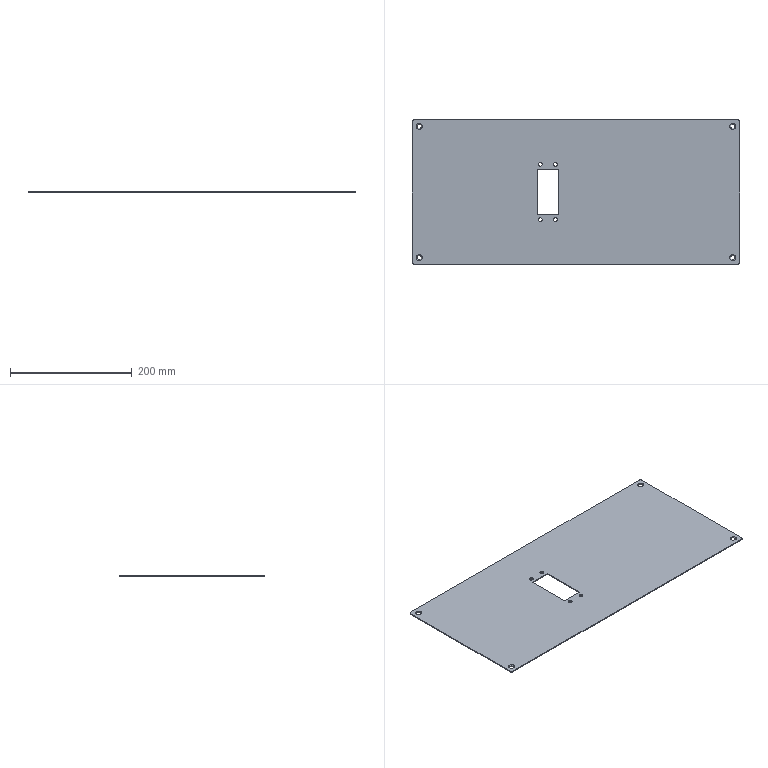Part | SolidWorks | features HoleWzd 2, Cut 1, Extrusion 1, Fillet 1, ICE 1 | 1 solid | 36 faces | box 538.2 x 238 x 1.5 mm | volume 187659 mm3 | cylinder 18 | plane 10 | cone 8 | commonest cylinder face diameters 6.4 x8 7.1 x6 6 x4
STEP:
#1=CARTESIAN_POINT('',(-25.62,94.068,-1.5));
#2=VERTEX_POINT('',#1);
#3=CARTESIAN_POINT('',(-19.22,94.068,-1.5));
#4=VERTEX_POINT('',#3);
#5=CARTESIAN_POINT('',(-22.42,94.068,-1.5));
#6=DIRECTION('',(0.,0.,1.));
#7=DIRECTION('',(1.,0.,0.));
#8=AXIS2_PLACEMENT_3D('',#5,#6,#7);
#9=CIRCLE('',#8,3.2);
#10=EDGE_CURVE('',#2,#4,#9,.T.);
#11=ORIENTED_EDGE('',*,*,#10,.F.);
#12=CARTESIAN_POINT('',(-25.62,94.068,0.));
#13=VERTEX_POINT('',#12);
#14=CARTESIAN_POINT('',(-25.62,94.068,-1.5));
#15=DIRECTION('',(0.,0.,1.));
#16=VECTOR('',#15,1000.);
#17=LINE('',#14,#16);
#18=EDGE_CURVE('',#2,#13,#17,.T.);
#19=ORIENTED_EDGE('',*,*,#18,.T.);
#20=CARTESIAN_POINT('',(-19.22,94.068,0.));
#21=VERTEX_POINT('',#20);
#22=CARTESIAN_POINT('',(-22.42,94.068,0.));
#23=DIRECTION('',(0.,0.,1.));
#24=DIRECTION('',(1.,0.,0.));
#25=AXIS2_PLACEMENT_3D('',#22,#23,#24);
#26=CIRCLE('',#25,3.2);
#27=EDGE_CURVE('',#13,#21,#26,.T.);
#28=ORIENTED_EDGE('',*,*,#27,.T.);
#29=CARTESIAN_POINT('',(-19.22,94.068,-1.5));
#30=DIRECTION('',(0.,0.,1.));
#31=VECTOR('',#30,1000.);
#32=LINE('',#29,#31);
#33=EDGE_CURVE('',#4,#21,#32,.T.);
#34=ORIENTED_EDGE('',*,*,#33,.F.);
#35=EDGE_LOOP('',(#11,#19,#28,#34));
#36=FACE_OUTER_BOUND('',#35,.T.);
#37=CARTESIAN_POINT('',(-22.42,94.068,-1.5));
#38=DIRECTION('',(0.,0.,1.));
#39=DIRECTION('',(1.,0.,0.));
#40=AXIS2_PLACEMENT_3D('',#37,#38,#39);
#41=CYLINDRICAL_SURFACE('',#40,3.2);
#42=ADVANCED_FACE('',(#36),#41,.F.);
#43=CARTESIAN_POINT('',(-0.6198,185.068,-1.5));
#44=VERTEX_POINT('',#43);
#45=CARTESIAN_POINT('',(5.78,185.068,-1.5));
#46=VERTEX_POINT('',#45);
#47=CARTESIAN_POINT('',(2.58,185.068,-1.5));
#48=DIRECTION('',(0.,0.,1.));
#49=DIRECTION('',(1.,0.,0.));
#50=AXIS2_PLACEMENT_3D('',#47,#48,#49);
#51=CIRCLE('',#50,3.2);
#52=EDGE_CURVE('',#44,#46,#51,.T.);
#53=ORIENTED_EDGE('',*,*,#52,.F.);
#54=CARTESIAN_POINT('',(-0.6198,185.068,0.));
#55=VERTEX_POINT('',#54);
#56=CARTESIAN_POINT('',(-0.6198,185.068,-1.5));
#57=DIRECTION('',(0.,0.,1.));
#58=VECTOR('',#57,1000.);
#59=LINE('',#56,#58);
#60=EDGE_CURVE('',#44,#55,#59,.T.);
#61=ORIENTED_EDGE('',*,*,#60,.T.);
#62=CARTESIAN_POINT('',(5.78,185.068,0.));
#63=VERTEX_POINT('',#62);
#64=CARTESIAN_POINT('',(2.58,185.068,0.));
#65=DIRECTION('',(0.,0.,1.));
#66=DIRECTION('',(1.,0.,0.));
#67=AXIS2_PLACEMENT_3D('',#64,#65,#66);
#68=CIRCLE('',#67,3.2);
#69=EDGE_CURVE('',#55,#63,#68,.T.);
#70=ORIENTED_EDGE('',*,*,#69,.T.);
#71=CARTESIAN_POINT('',(5.78,185.068,-1.5));
#72=DIRECTION('',(0.,0.,1.));
#73=VECTOR('',#72,1000.);
#74=LINE('',#71,#73);
#75=EDGE_CURVE('',#46,#63,#74,.T.);
#76=ORIENTED_EDGE('',*,*,#75,.F.);
#77=EDGE_LOOP('',(#53,#61,#70,#76));
#78=FACE_OUTER_BOUND('',#77,.T.);
#79=CARTESIAN_POINT('',(2.58,185.068,-1.5));
#80=DIRECTION('',(0.,0.,1.));
#81=DIRECTION('',(1.,0.,0.));
#82=AXIS2_PLACEMENT_3D('',#79,#80,#81);
#83=CYLINDRICAL_SURFACE('',#82,3.2);
#84=ADVANCED_FACE('',(#78),#83,.F.);
#85=CARTESIAN_POINT('',(-25.62,185.068,-1.5));
#86=VERTEX_POINT('',#85);
#87=CARTESIAN_POINT('',(-19.22,185.068,-1.5));
#88=VERTEX_POINT('',#87);
#89=CARTESIAN_POINT('',(-22.42,185.068,-1.5));
#90=DIRECTION('',(0.,0.,1.));
#91=DIRECTION('',(1.,0.,0.));
#92=AXIS2_PLACEMENT_3D('',#89,#90,#91);
#93=CIRCLE('',#92,3.2);
#94=EDGE_CURVE('',#86,#88,#93,.T.);
#95=ORIENTED_EDGE('',*,*,#94,.F.);
#96=CARTESIAN_POINT('',(-25.62,185.068,0.));
#97=VERTEX_POINT('',#96);
#98=CARTESIAN_POINT('',(-25.62,185.068,-1.5));
#99=DIRECTION('',(0.,0.,1.));
#100=VECTOR('',#99,1000.);
#101=LINE('',#98,#100);
#102=EDGE_CURVE('',#86,#97,#101,.T.);
#103=ORIENTED_EDGE('',*,*,#102,.T.);
#104=CARTESIAN_POINT('',(-19.22,185.068,0.));
#105=VERTEX_POINT('',#104);
#106=CARTESIAN_POINT('',(-22.42,185.068,0.));
#107=DIRECTION('',(0.,0.,1.));
#108=DIRECTION('',(1.,0.,0.));
#109=AXIS2_PLACEMENT_3D('',#106,#107,#108);
#110=CIRCLE('',#109,3.2);
#111=EDGE_CURVE('',#97,#105,#110,.T.);
#112=ORIENTED_EDGE('',*,*,#111,.T.);
#113=CARTESIAN_POINT('',(-19.22,185.068,-1.5));
#114=DIRECTION('',(0.,0.,1.));
#115=VECTOR('',#114,1000.);
#116=LINE('',#113,#115);
#117=EDGE_CURVE('',#88,#105,#116,.T.);
#118=ORIENTED_EDGE('',*,*,#117,.F.);
#119=EDGE_LOOP('',(#95,#103,#112,#118));
#120=FACE_OUTER_BOUND('',#119,.T.);
#121=CARTESIAN_POINT('',(-22.42,185.068,-1.5));
#122=DIRECTION('',(0.,0.,1.));
#123=DIRECTION('',(1.,0.,0.));
#124=AXIS2_PLACEMENT_3D('',#121,#122,#123);
#125=CYLINDRICAL_SURFACE('',#124,3.2);
#126=ADVANCED_FACE('',(#120),#125,.F.);
#127=CARTESIAN_POINT('',(-0.6198,94.068,-1.5));
#128=VERTEX_POINT('',#127);
#129=CARTESIAN_POINT('',(5.78,94.068,-1.5));
#130=VERTEX_POINT('',#129);
#131=CARTESIAN_POINT('',(2.58,94.068,-1.5));
#132=DIRECTION('',(0.,0.,1.));
#133=DIRECTION('',(1.,0.,0.));
#134=AXIS2_PLACEMENT_3D('',#131,#132,#133);
#135=CIRCLE('',#134,3.2);
#136=EDGE_CURVE('',#128,#130,#135,.T.);
#137=ORIENTED_EDGE('',*,*,#136,.F.);
#138=CARTESIAN_POINT('',(-0.6198,94.068,0.));
#139=VERTEX_POINT('',#138);
#140=CARTESIAN_POINT('',(-0.6198,94.068,-1.5));
#141=DIRECTION('',(0.,0.,1.));
#142=VECTOR('',#141,1000.);
#143=LINE('',#140,#142);
#144=EDGE_CURVE('',#128,#139,#143,.T.);
#145=ORIENTED_EDGE('',*,*,#144,.T.);
#146=CARTESIAN_POINT('',(5.78,94.068,0.));
#147=VERTEX_POINT('',#146);
#148=CARTESIAN_POINT('',(2.58,94.068,0.));
#149=DIRECTION('',(0.,0.,1.));
#150=DIRECTION('',(1.,0.,0.));
#151=AXIS2_PLACEMENT_3D('',#148,#149,#150);
#152=CIRCLE('',#151,3.2);
#153=EDGE_CURVE('',#139,#147,#152,.T.);
#154=ORIENTED_EDGE('',*,*,#153,.T.);
#155=CARTESIAN_POINT('',(5.78,94.068,-1.5));
#156=DIRECTION('',(0.,0.,1.));
#157=VECTOR('',#156,1000.);
#158=LINE('',#155,#157);
#159=EDGE_CURVE('',#130,#147,#158,.T.);
#160=ORIENTED_EDGE('',*,*,#159,.F.);
#161=EDGE_LOOP('',(#137,#145,#154,#160));
#162=FACE_OUTER_BOUND('',#161,.T.);
#163=CARTESIAN_POINT('',(2.58,94.068,-1.5));
#164=DIRECTION('',(0.,0.,1.));
#165=DIRECTION('',(1.,0.,0.));
#166=AXIS2_PLACEMENT_3D('',#163,#164,#165);
#167=CYLINDRICAL_SURFACE('',#166,3.2);
#168=ADVANCED_FACE('',(#162),#167,.F.);
#169=CARTESIAN_POINT('',(291.03,247.568,-1.4));
#170=VERTEX_POINT('',#169);
#171=CARTESIAN_POINT('',(298.13,247.568,-1.4));
#172=VERTEX_POINT('',#171);
#173=CARTESIAN_POINT('',(294.58,247.568,-1.4));
#174=DIRECTION('',(0.,0.,1.));
#175=DIRECTION('',(1.,0.,0.));
#176=AXIS2_PLACEMENT_3D('',#173,#174,#175);
#177=CIRCLE('',#176,3.55);
#178=EDGE_CURVE('',#170,#172,#177,.T.);
#179=ORIENTED_EDGE('',*,*,#178,.F.);
#180=CARTESIAN_POINT('',(289.63,247.568,0.));
#181=VERTEX_POINT('',#180);
#182=CARTESIAN_POINT('',(289.63,247.568,0.));
#183=DIRECTION('',(-0.7071,0.,0.7071));
#184=VECTOR('',#183,1000.);
#185=LINE('',#182,#184);
#186=EDGE_CURVE('',#170,#181,#185,.T.);
#187=ORIENTED_EDGE('',*,*,#186,.T.);
#188=CARTESIAN_POINT('',(299.53,247.568,0.));
#189=VERTEX_POINT('',#188);
#190=CARTESIAN_POINT('',(294.58,247.568,0.));
#191=DIRECTION('',(0.,0.,1.));
#192=DIRECTION('',(1.,0.,0.));
#193=AXIS2_PLACEMENT_3D('',#190,#191,#192);
#194=CIRCLE('',#193,4.95);
#195=EDGE_CURVE('',#181,#189,#194,.T.);
#196=ORIENTED_EDGE('',*,*,#195,.T.);
#197=CARTESIAN_POINT('',(299.53,247.568,0.));
#198=DIRECTION('',(0.7071,0.,0.7071));
#199=VECTOR('',#198,1000.);
#200=LINE('',#197,#199);
#201=EDGE_CURVE('',#172,#189,#200,.T.);
#202=ORIENTED_EDGE('',*,*,#201,.F.);
#203=EDGE_LOOP('',(#179,#187,#196,#202));
#204=FACE_OUTER_BOUND('',#203,.T.);
#205=CARTESIAN_POINT('',(294.58,247.568,0.));
#206=DIRECTION('',(0.,0.,1.));
#207=DIRECTION('',(1.,0.,0.));
#208=AXIS2_PLACEMENT_3D('',#205,#206,#207);
#209=CONICAL_SURFACE('',#208,4.95,0.7854);
#210=ADVANCED_FACE('',(#204),#209,.F.);
#211=CARTESIAN_POINT('',(291.03,247.568,-1.5));
#212=VERTEX_POINT('',#211);
#213=CARTESIAN_POINT('',(298.13,247.568,-1.5));
#214=VERTEX_POINT('',#213);
#215=CARTESIAN_POINT('',(294.58,247.568,-1.5));
#216=DIRECTION('',(0.,0.,1.));
#217=DIRECTION('',(1.,0.,0.));
#218=AXIS2_PLACEMENT_3D('',#215,#216,#217);
#219=CIRCLE('',#218,3.55);
#220=EDGE_CURVE('',#212,#214,#219,.T.);
#221=ORIENTED_EDGE('',*,*,#220,.F.);
#222=CARTESIAN_POINT('',(291.03,247.568,0.));
#223=DIRECTION('',(0.,0.,1.));
#224=VECTOR('',#223,1000.);
#225=LINE('',#222,#224);
#226=EDGE_CURVE('',#212,#170,#225,.T.);
#227=ORIENTED_EDGE('',*,*,#226,.T.);
#228=ORIENTED_EDGE('',*,*,#178,.T.);
#229=CARTESIAN_POINT('',(298.13,247.568,0.));
#230=DIRECTION('',(0.,0.,1.));
#231=VECTOR('',#230,1000.);
#232=LINE('',#229,#231);
#233=EDGE_CURVE('',#214,#172,#232,.T.);
#234=ORIENTED_EDGE('',*,*,#233,.F.);
#235=EDGE_LOOP('',(#221,#227,#228,#234));
#236=FACE_OUTER_BOUND('',#235,.T.);
#237=CARTESIAN_POINT('',(294.58,247.568,0.));
#238=DIRECTION('',(0.,0.,1.));
#239=DIRECTION('',(1.,0.,0.));
#240=AXIS2_PLACEMENT_3D('',#237,#238,#239);
#241=CYLINDRICAL_SURFACE('',#240,3.55);
#242=ADVANCED_FACE('',(#236),#241,.F.);
#243=CARTESIAN_POINT('',(291.03,31.568,-1.4));
#244=VERTEX_POINT('',#243);
#245=CARTESIAN_POINT('',(298.13,31.568,-1.4));
#246=VERTEX_POINT('',#245);
#247=CARTESIAN_POINT('',(294.58,31.568,-1.4));
#248=DIRECTION('',(0.,0.,1.));
#249=DIRECTION('',(1.,0.,0.));
#250=AXIS2_PLACEMENT_3D('',#247,#248,#249);
#251=CIRCLE('',#250,3.55);
#252=EDGE_CURVE('',#244,#246,#251,.T.);
#253=ORIENTED_EDGE('',*,*,#252,.F.);
#254=CARTESIAN_POINT('',(289.63,31.568,0.));
#255=VERTEX_POINT('',#254);
#256=CARTESIAN_POINT('',(289.63,31.568,0.));
#257=DIRECTION('',(-0.7071,0.,0.7071));
#258=VECTOR('',#257,1000.);
#259=LINE('',#256,#258);
#260=EDGE_CURVE('',#244,#255,#259,.T.);
#261=ORIENTED_EDGE('',*,*,#260,.T.);
#262=CARTESIAN_POINT('',(299.53,31.568,0.));
#263=VERTEX_POINT('',#262);
#264=CARTESIAN_POINT('',(294.58,31.568,0.));
#265=DIRECTION('',(0.,0.,1.));
#266=DIRECTION('',(1.,0.,0.));
#267=AXIS2_PLACEMENT_3D('',#264,#265,#266);
#268=CIRCLE('',#267,4.95);
#269=EDGE_CURVE('',#255,#263,#268,.T.);
#270=ORIENTED_EDGE('',*,*,#269,.T.);
#271=CARTESIAN_POINT('',(299.53,31.568,0.));
#272=DIRECTION('',(0.7071,0.,0.7071));
#273=VECTOR('',#272,1000.);
#274=LINE('',#271,#273);
#275=EDGE_CURVE('',#246,#263,#274,.T.);
#276=ORIENTED_EDGE('',*,*,#275,.F.);
#277=EDGE_LOOP('',(#253,#261,#270,#276));
#278=FACE_OUTER_BOUND('',#277,.T.);
#279=CARTESIAN_POINT('',(294.58,31.568,0.));
#280=DIRECTION('',(0.,0.,1.));
#281=DIRECTION('',(1.,0.,0.));
#282=AXIS2_PLACEMENT_3D('',#279,#280,#281);
#283=CONICAL_SURFACE('',#282,4.95,0.7854);
#284=ADVANCED_FACE('',(#278),#283,.F.);
#285=CARTESIAN_POINT('',(291.03,31.568,-1.5));
#286=VERTEX_POINT('',#285);
#287=CARTESIAN_POINT('',(298.13,31.568,-1.5));
#288=VERTEX_POINT('',#287);
#289=CARTESIAN_POINT('',(294.58,31.568,-1.5));
#290=DIRECTION('',(0.,0.,1.));
#291=DIRECTION('',(1.,0.,0.));
#292=AXIS2_PLACEMENT_3D('',#289,#290,#291);
#293=CIRCLE('',#292,3.55);
#294=EDGE_CURVE('',#286,#288,#293,.T.);
#295=ORIENTED_EDGE('',*,*,#294,.F.);
#296=CARTESIAN_POINT('',(291.03,31.568,0.));
#297=DIRECTION('',(0.,0.,1.));
#298=VECTOR('',#297,1000.);
#299=LINE('',#296,#298);
#300=EDGE_CURVE('',#286,#244,#299,.T.);
#301=ORIENTED_EDGE('',*,*,#300,.T.);
#302=ORIENTED_EDGE('',*,*,#252,.T.);
#303=CARTESIAN_POINT('',(298.13,31.568,0.));
#304=DIRECTION('',(0.,0.,1.));
#305=VECTOR('',#304,1000.);
#306=LINE('',#303,#305);
#307=EDGE_CURVE('',#288,#246,#306,.T.);
#308=ORIENTED_EDGE('',*,*,#307,.F.);
#309=EDGE_LOOP('',(#295,#301,#302,#308));
#310=FACE_OUTER_BOUND('',#309,.T.);
#311=CARTESIAN_POINT('',(294.58,31.568,0.));
#312=DIRECTION('',(0.,0.,1.));
#313=DIRECTION('',(1.,0.,0.));
#314=AXIS2_PLACEMENT_3D('',#311,#312,#313);
#315=CYLINDRICAL_SURFACE('',#314,3.55);
#316=ADVANCED_FACE('',(#310),#315,.F.);
#317=CARTESIAN_POINT('',(-225.17,247.568,-1.4));
#318=VERTEX_POINT('',#317);
#319=CARTESIAN_POINT('',(-218.07,247.568,-1.4));
#320=VERTEX_POINT('',#319);
#321=CARTESIAN_POINT('',(-221.62,247.568,-1.4));
#322=DIRECTION('',(0.,0.,1.));
#323=DIRECTION('',(1.,0.,0.));
#324=AXIS2_PLACEMENT_3D('',#321,#322,#323);
#325=CIRCLE('',#324,3.55);
#326=EDGE_CURVE('',#318,#320,#325,.T.);
#327=ORIENTED_EDGE('',*,*,#326,.F.);
#328=CARTESIAN_POINT('',(-226.57,247.568,0.));
#329=VERTEX_POINT('',#328);
#330=CARTESIAN_POINT('',(-226.57,247.568,0.));
#331=DIRECTION('',(-0.7071,0.,0.7071));
#332=VECTOR('',#331,1000.);
#333=LINE('',#330,#332);
#334=EDGE_CURVE('',#318,#329,#333,.T.);
#335=ORIENTED_EDGE('',*,*,#334,.T.);
#336=CARTESIAN_POINT('',(-216.67,247.568,0.));
#337=VERTEX_POINT('',#336);
#338=CARTESIAN_POINT('',(-221.62,247.568,0.));
#339=DIRECTION('',(0.,0.,1.));
#340=DIRECTION('',(1.,0.,0.));
#341=AXIS2_PLACEMENT_3D('',#338,#339,#340);
#342=CIRCLE('',#341,4.95);
#343=EDGE_CURVE('',#329,#337,#342,.T.);
#344=ORIENTED_EDGE('',*,*,#343,.T.);
#345=CARTESIAN_POINT('',(-216.67,247.568,0.));
#346=DIRECTION('',(0.7071,0.,0.7071));
#347=VECTOR('',#346,1000.);
#348=LINE('',#345,#347);
#349=EDGE_CURVE('',#320,#337,#348,.T.);
#350=ORIENTED_EDGE('',*,*,#349,.F.);
#351=EDGE_LOOP('',(#327,#335,#344,#350));
#352=FACE_OUTER_BOUND('',#351,.T.);
#353=CARTESIAN_POINT('',(-221.62,247.568,0.));
#354=DIRECTION('',(0.,0.,1.));
#355=DIRECTION('',(1.,0.,0.));
#356=AXIS2_PLACEMENT_3D('',#353,#354,#355);
#357=CONICAL_SURFACE('',#356,4.95,0.7854);
#358=ADVANCED_FACE('',(#352),#357,.F.);
#359=CARTESIAN_POINT('',(-225.17,247.568,-1.5));
#360=VERTEX_POINT('',#359);
#361=CARTESIAN_POINT('',(-218.07,247.568,-1.5));
#362=VERTEX_POINT('',#361);
#363=CARTESIAN_POINT('',(-221.62,247.568,-1.5));
#364=DIRECTION('',(0.,0.,1.));
#365=DIRECTION('',(1.,0.,0.));
#366=AXIS2_PLACEMENT_3D('',#363,#364,#365);
#367=CIRCLE('',#366,3.55);
#368=EDGE_CURVE('',#360,#362,#367,.T.);
#369=ORIENTED_EDGE('',*,*,#368,.F.);
#370=CARTESIAN_POINT('',(-225.17,247.568,0.));
#371=DIRECTION('',(0.,0.,1.));
#372=VECTOR('',#371,1000.);
#373=LINE('',#370,#372);
#374=EDGE_CURVE('',#360,#318,#373,.T.);
#375=ORIENTED_EDGE('',*,*,#374,.T.);
#376=ORIENTED_EDGE('',*,*,#326,.T.);
#377=CARTESIAN_POINT('',(-218.07,247.568,0.));
#378=DIRECTION('',(0.,0.,1.));
#379=VECTOR('',#378,1000.);
#380=LINE('',#377,#379);
#381=EDGE_CURVE('',#362,#320,#380,.T.);
#382=ORIENTED_EDGE('',*,*,#381,.F.);
#383=EDGE_LOOP('',(#369,#375,#376,#382));
#384=FACE_OUTER_BOUND('',#383,.T.);
#385=CARTESIAN_POINT('',(-221.62,247.568,0.));
#386=DIRECTION('',(0.,0.,1.));
#387=DIRECTION('',(1.,0.,0.));
#388=AXIS2_PLACEMENT_3D('',#385,#386,#387);
#389=CYLINDRICAL_SURFACE('',#388,3.55);
#390=ADVANCED_FACE('',(#384),#389,.F.);
#391=CARTESIAN_POINT('',(-225.07,31.568,-1.5));
#392=VERTEX_POINT('',#391);
#393=CARTESIAN_POINT('',(-218.17,31.568,-1.5));
#394=VERTEX_POINT('',#393);
#395=CARTESIAN_POINT('',(-221.62,31.568,-1.5));
#396=DIRECTION('',(0.,0.,1.));
#397=DIRECTION('',(1.,0.,0.));
#398=AXIS2_PLACEMENT_3D('',#395,#396,#397);
#399=CIRCLE('',#398,3.45);
#400=EDGE_CURVE('',#392,#394,#399,.T.);
#401=ORIENTED_EDGE('',*,*,#400,.F.);
#402=CARTESIAN_POINT('',(-226.57,31.568,0.));
#403=VERTEX_POINT('',#402);
#404=CARTESIAN_POINT('',(-226.57,31.568,0.));
#405=DIRECTION('',(-0.7071,0.,0.7071));
#406=VECTOR('',#405,1000.);
#407=LINE('',#404,#406);
#408=EDGE_CURVE('',#392,#403,#407,.T.);
#409=ORIENTED_EDGE('',*,*,#408,.T.);
#410=CARTESIAN_POINT('',(-216.67,31.568,0.));
#411=VERTEX_POINT('',#410);
#412=CARTESIAN_POINT('',(-221.62,31.568,0.));
#413=DIRECTION('',(0.,0.,1.));
#414=DIRECTION('',(1.,0.,0.));
#415=AXIS2_PLACEMENT_3D('',#412,#413,#414);
#416=CIRCLE('',#415,4.95);
#417=EDGE_CURVE('',#403,#411,#416,.T.);
#418=ORIENTED_EDGE('',*,*,#417,.T.);
#419=CARTESIAN_POINT('',(-216.67,31.568,0.));
#420=DIRECTION('',(0.7071,0.,0.7071));
#421=VECTOR('',#420,1000.);
#422=LINE('',#419,#421);
#423=EDGE_CURVE('',#394,#411,#422,.T.);
#424=ORIENTED_EDGE('',*,*,#423,.F.);
#425=EDGE_LOOP('',(#401,#409,#418,#424));
#426=FACE_OUTER_BOUND('',#425,.T.);
#427=CARTESIAN_POINT('',(-221.62,31.568,0.));
#428=DIRECTION('',(0.,0.,1.));
#429=DIRECTION('',(1.,0.,0.));
#430=AXIS2_PLACEMENT_3D('',#427,#428,#429);
#431=CONICAL_SURFACE('',#430,4.95,0.7854);
#432=ADVANCED_FACE('',(#426),#431,.F.);
#433=CARTESIAN_POINT('',(-232.62,255.568,-1.5));
#434=VERTEX_POINT('',#433);
#435=CARTESIAN_POINT('',(-232.62,23.568,-1.5));
#436=VERTEX_POINT('',#435);
#437=CARTESIAN_POINT('',(-232.62,258.568,-1.5));
#438=DIRECTION('',(0.,-1.,0.));
#439=VECTOR('',#438,1000.);
#440=LINE('',#437,#439);
#441=EDGE_CURVE('',#434,#436,#440,.T.);
#442=ORIENTED_EDGE('',*,*,#441,.T.);
#443=CARTESIAN_POINT('',(-232.62,23.568,0.));
#444=VERTEX_POINT('',#443);
#445=CARTESIAN_POINT('',(-232.62,23.568,-1.5));
#446=DIRECTION('',(0.,0.,1.));
#447=VECTOR('',#446,1000.);
#448=LINE('',#445,#447);
#449=EDGE_CURVE('',#436,#444,#448,.T.);
#450=ORIENTED_EDGE('',*,*,#449,.T.);
#451=CARTESIAN_POINT('',(-232.62,255.568,0.));
#452=VERTEX_POINT('',#451);
#453=CARTESIAN_POINT('',(-232.62,258.568,0.));
#454=DIRECTION('',(0.,-1.,0.));
#455=VECTOR('',#454,1000.);
#456=LINE('',#453,#455);
#457=EDGE_CURVE('',#452,#444,#456,.T.);
#458=ORIENTED_EDGE('',*,*,#457,.F.);
#459=CARTESIAN_POINT('',(-232.62,255.568,-1.5));
#460=DIRECTION('',(0.,0.,-1.));
#461=VECTOR('',#460,1000.);
#462=LINE('',#459,#461);
#463=EDGE_CURVE('',#452,#434,#462,.T.);
#464=ORIENTED_EDGE('',*,*,#463,.T.);
#465=EDGE_LOOP('',(#442,#450,#458,#464));
#466=FACE_OUTER_BOUND('',#465,.T.);
#467=CARTESIAN_POINT('',(-232.62,258.568,-1.5));
#468=DIRECTION('',(-1.,0.,0.));
#469=DIRECTION('',(0.,0.,1.));
#470=AXIS2_PLACEMENT_3D('',#467,#468,#469);
#471=PLANE('',#470);
#472=ADVANCED_FACE('',(#466),#471,.T.);
#473=CARTESIAN_POINT('',(302.58,258.568,0.));
#474=VERTEX_POINT('',#473);
#475=CARTESIAN_POINT('',(-229.62,258.568,0.));
#476=VERTEX_POINT('',#475);
#477=CARTESIAN_POINT('',(305.58,258.568,0.));
#478=DIRECTION('',(-1.,0.,0.));
#479=VECTOR('',#478,1000.);
#480=LINE('',#477,#479);
#481=EDGE_CURVE('',#474,#476,#480,.T.);
#482=ORIENTED_EDGE('',*,*,#481,.F.);
#483=CARTESIAN_POINT('',(302.58,258.568,-1.5));
#484=VERTEX_POINT('',#483);
#485=CARTESIAN_POINT('',(302.58,258.568,-1.5));
#486=DIRECTION('',(0.,0.,-1.));
#487=VECTOR('',#486,1000.);
#488=LINE('',#485,#487);
#489=EDGE_CURVE('',#474,#484,#488,.T.);
#490=ORIENTED_EDGE('',*,*,#489,.T.);
#491=CARTESIAN_POINT('',(-229.62,258.568,-1.5));
#492=VERTEX_POINT('',#491);
#493=CARTESIAN_POINT('',(305.58,258.568,-1.5));
#494=DIRECTION('',(-1.,0.,0.));
#495=VECTOR('',#494,1000.);
#496=LINE('',#493,#495);
#497=EDGE_CURVE('',#484,#492,#496,.T.);
#498=ORIENTED_EDGE('',*,*,#497,.T.);
#499=CARTESIAN_POINT('',(-229.62,258.568,-1.5));
#500=DIRECTION('',(0.,0.,1.));
#501=VECTOR('',#500,1000.);
#502=LINE('',#499,#501);
#503=EDGE_CURVE('',#492,#476,#502,.T.);
#504=ORIENTED_EDGE('',*,*,#503,.T.);
#505=EDGE_LOOP('',(#482,#490,#498,#504));
#506=FACE_OUTER_BOUND('',#505,.T.);
#507=CARTESIAN_POINT('',(305.58,258.568,-1.5));
#508=DIRECTION('',(0.,1.,0.));
#509=DIRECTION('',(-1.,0.,0.));
#510=AXIS2_PLACEMENT_3D('',#507,#508,#509);
#511=PLANE('',#510);
#512=ADVANCED_FACE('',(#506),#511,.T.);
#513=CARTESIAN_POINT('',(305.58,23.568,0.));
#514=VERTEX_POINT('',#513);
#515=CARTESIAN_POINT('',(305.58,255.568,0.));
#516=VERTEX_POINT('',#515);
#517=CARTESIAN_POINT('',(305.58,20.568,0.));
#518=DIRECTION('',(0.,1.,0.));
#519=VECTOR('',#518,1000.);
#520=LINE('',#517,#519);
#521=EDGE_CURVE('',#514,#516,#520,.T.);
#522=ORIENTED_EDGE('',*,*,#521,.F.);
#523=CARTESIAN_POINT('',(305.58,23.568,-1.5));
#524=VERTEX_POINT('',#523);
#525=CARTESIAN_POINT('',(305.58,23.568,-1.5));
#526=DIRECTION('',(0.,0.,-1.));
#527=VECTOR('',#526,1000.);
#528=LINE('',#525,#527);
#529=EDGE_CURVE('',#514,#524,#528,.T.);
#530=ORIENTED_EDGE('',*,*,#529,.T.);
#531=CARTESIAN_POINT('',(305.58,255.568,-1.5));
#532=VERTEX_POINT('',#531);
#533=CARTESIAN_POINT('',(305.58,20.568,-1.5));
#534=DIRECTION('',(0.,1.,0.));
#535=VECTOR('',#534,1000.);
#536=LINE('',#533,#535);
#537=EDGE_CURVE('',#524,#532,#536,.T.);
#538=ORIENTED_EDGE('',*,*,#537,.T.);
#539=CARTESIAN_POINT('',(305.58,255.568,-1.5));
#540=DIRECTION('',(0.,0.,1.));
#541=VECTOR('',#540,1000.);
#542=LINE('',#539,#541);
#543=EDGE_CURVE('',#532,#516,#542,.T.);
#544=ORIENTED_EDGE('',*,*,#543,.T.);
#545=EDGE_LOOP('',(#522,#530,#538,#544));
#546=FACE_OUTER_BOUND('',#545,.T.);
#547=CARTESIAN_POINT('',(305.58,20.568,-1.5));
#548=DIRECTION('',(1.,0.,0.));
#549=DIRECTION('',(0.,0.,-1.));
#550=AXIS2_PLACEMENT_3D('',#547,#548,#549);
#551=PLANE('',#550);
#552=ADVANCED_FACE('',(#546),#551,.T.);
#553=CARTESIAN_POINT('',(-229.62,20.568,-1.5));
#554=VERTEX_POINT('',#553);
#555=CARTESIAN_POINT('',(302.58,20.568,-1.5));
#556=VERTEX_POINT('',#555);
#557=CARTESIAN_POINT('',(-232.62,20.568,-1.5));
#558=DIRECTION('',(1.,0.,0.));
#559=VECTOR('',#558,1000.);
#560=LINE('',#557,#559);
#561=EDGE_CURVE('',#554,#556,#560,.T.);
#562=ORIENTED_EDGE('',*,*,#561,.T.);
#563=CARTESIAN_POINT('',(302.58,20.568,0.));
#564=VERTEX_POINT('',#563);
#565=CARTESIAN_POINT('',(302.58,20.568,-1.5));
#566=DIRECTION('',(0.,0.,1.));
#567=VECTOR('',#566,1000.);
#568=LINE('',#565,#567);
#569=EDGE_CURVE('',#556,#564,#568,.T.);
#570=ORIENTED_EDGE('',*,*,#569,.T.);
#571=CARTESIAN_POINT('',(-229.62,20.568,0.));
#572=VERTEX_POINT('',#571);
#573=CARTESIAN_POINT('',(-232.62,20.568,0.));
#574=DIRECTION('',(1.,0.,0.));
#575=VECTOR('',#574,1000.);
#576=LINE('',#573,#575);
#577=EDGE_CURVE('',#572,#564,#576,.T.);
#578=ORIENTED_EDGE('',*,*,#577,.F.);
#579=CARTESIAN_POINT('',(-229.62,20.568,-1.5));
#580=DIRECTION('',(0.,0.,-1.));
#581=VECTOR('',#580,1000.);
#582=LINE('',#579,#581);
#583=EDGE_CURVE('',#572,#554,#582,.T.);
#584=ORIENTED_EDGE('',*,*,#583,.T.);
#585=EDGE_LOOP('',(#562,#570,#578,#584));
#586=FACE_OUTER_BOUND('',#585,.T.);
#587=CARTESIAN_POINT('',(-232.62,20.568,-1.5));
#588=DIRECTION('',(0.,-1.,0.));
#589=DIRECTION('',(1.,0.,0.));
#590=AXIS2_PLACEMENT_3D('',#587,#588,#589);
#591=PLANE('',#590);
#592=ADVANCED_FACE('',(#586),#591,.T.);
#593=CARTESIAN_POINT('',(-22.42,94.068,-1.5));
#594=DIRECTION('',(0.,0.,1.));
#595=DIRECTION('',(1.,0.,0.));
#596=AXIS2_PLACEMENT_3D('',#593,#594,#595);
#597=CIRCLE('',#596,3.2);
#598=EDGE_CURVE('',#4,#2,#597,.T.);
#599=ORIENTED_EDGE('',*,*,#598,.T.);
#600=ORIENTED_EDGE('',*,*,#10,.T.);
#601=EDGE_LOOP('',(#599,#600));
#602=FACE_BOUND('',#601,.T.);
#603=CARTESIAN_POINT('',(2.58,185.068,-1.5));
#604=DIRECTION('',(0.,0.,1.));
#605=DIRECTION('',(1.,0.,0.));
#606=AXIS2_PLACEMENT_3D('',#603,#604,#605);
#607=CIRCLE('',#606,3.2);
#608=EDGE_CURVE('',#46,#44,#607,.T.);
#609=ORIENTED_EDGE('',*,*,#608,.T.);
#610=ORIENTED_EDGE('',*,*,#52,.T.);
#611=EDGE_LOOP('',(#609,#610));
#612=FACE_BOUND('',#611,.T.);
#613=CARTESIAN_POINT('',(-22.42,185.068,-1.5));
#614=DIRECTION('',(0.,0.,1.));
#615=DIRECTION('',(1.,0.,0.));
#616=AXIS2_PLACEMENT_3D('',#613,#614,#615);
#617=CIRCLE('',#616,3.2);
#618=EDGE_CURVE('',#88,#86,#617,.T.);
#619=ORIENTED_EDGE('',*,*,#618,.T.);
#620=ORIENTED_EDGE('',*,*,#94,.T.);
#621=EDGE_LOOP('',(#619,#620));
#622=FACE_BOUND('',#621,.T.);
#623=CARTESIAN_POINT('',(2.58,94.068,-1.5));
#624=DIRECTION('',(0.,0.,1.));
#625=DIRECTION('',(1.,0.,0.));
#626=AXIS2_PLACEMENT_3D('',#623,#624,#625);
#627=CIRCLE('',#626,3.2);
#628=EDGE_CURVE('',#130,#128,#627,.T.);
#629=ORIENTED_EDGE('',*,*,#628,.T.);
#630=ORIENTED_EDGE('',*,*,#136,.T.);
#631=EDGE_LOOP('',(#629,#630));
#632=FACE_BOUND('',#631,.T.);
#633=CARTESIAN_POINT('',(-27.42,102.068,-1.5));
#634=VERTEX_POINT('',#633);
#635=CARTESIAN_POINT('',(7.58,102.068,-1.5));
#636=VERTEX_POINT('',#635);
#637=CARTESIAN_POINT('',(7.58,102.068,-1.5));
#638=DIRECTION('',(1.,0.,0.));
#639=VECTOR('',#638,1000.);
#640=LINE('',#637,#639);
#641=EDGE_CURVE('',#634,#636,#640,.T.);
#642=ORIENTED_EDGE('',*,*,#641,.T.);
#643=CARTESIAN_POINT('',(7.58,177.068,-1.5));
#644=VERTEX_POINT('',#643);
#645=CARTESIAN_POINT('',(7.58,102.068,-1.5));
#646=DIRECTION('',(0.,1.,0.));
#647=VECTOR('',#646,1000.);
#648=LINE('',#645,#647);
#649=EDGE_CURVE('',#636,#644,#648,.T.);
#650=ORIENTED_EDGE('',*,*,#649,.T.);
#651=CARTESIAN_POINT('',(-27.42,177.068,-1.5));
#652=VERTEX_POINT('',#651);
#653=CARTESIAN_POINT('',(7.58,177.068,-1.5));
#654=DIRECTION('',(-1.,0.,0.));
#655=VECTOR('',#654,1000.);
#656=LINE('',#653,#655);
#657=EDGE_CURVE('',#644,#652,#656,.T.);
#658=ORIENTED_EDGE('',*,*,#657,.T.);
#659=CARTESIAN_POINT('',(-27.42,102.068,-1.5));
#660=DIRECTION('',(0.,-1.,0.));
#661=VECTOR('',#660,1000.);
#662=LINE('',#659,#661);
#663=EDGE_CURVE('',#652,#634,#662,.T.);
#664=ORIENTED_EDGE('',*,*,#663,.T.);
#665=EDGE_LOOP('',(#642,#650,#658,#664));
#666=FACE_BOUND('',#665,.T.);
#667=CARTESIAN_POINT('',(294.58,247.568,-1.5));
#668=DIRECTION('',(0.,0.,1.));
#669=DIRECTION('',(1.,0.,0.));
#670=AXIS2_PLACEMENT_3D('',#667,#668,#669);
#671=CIRCLE('',#670,3.55);
#672=EDGE_CURVE('',#214,#212,#671,.T.);
#673=ORIENTED_EDGE('',*,*,#672,.T.);
#674=ORIENTED_EDGE('',*,*,#220,.T.);
#675=EDGE_LOOP('',(#673,#674));
#676=FACE_BOUND('',#675,.T.);
#677=CARTESIAN_POINT('',(294.58,31.568,-1.5));
#678=DIRECTION('',(0.,0.,1.));
#679=DIRECTION('',(1.,0.,0.));
#680=AXIS2_PLACEMENT_3D('',#677,#678,#679);
#681=CIRCLE('',#680,3.55);
#682=EDGE_CURVE('',#288,#286,#681,.T.);
#683=ORIENTED_EDGE('',*,*,#682,.T.);
#684=ORIENTED_EDGE('',*,*,#294,.T.);
#685=EDGE_LOOP('',(#683,#684));
#686=FACE_BOUND('',#685,.T.);
#687=CARTESIAN_POINT('',(-221.62,247.568,-1.5));
#688=DIRECTION('',(0.,0.,1.));
#689=DIRECTION('',(1.,0.,0.));
#690=AXIS2_PLACEMENT_3D('',#687,#688,#689);
#691=CIRCLE('',#690,3.55);
#692=EDGE_CURVE('',#362,#360,#691,.T.);
#693=ORIENTED_EDGE('',*,*,#692,.T.);
#694=ORIENTED_EDGE('',*,*,#368,.T.);
#695=EDGE_LOOP('',(#693,#694));
#696=FACE_BOUND('',#695,.T.);
#697=CARTESIAN_POINT('',(-221.62,31.568,-1.5));
#698=DIRECTION('',(0.,0.,1.));
#699=DIRECTION('',(1.,0.,0.));
#700=AXIS2_PLACEMENT_3D('',#697,#698,#699);
#701=CIRCLE('',#700,3.45);
#702=EDGE_CURVE('',#394,#392,#701,.T.);
#703=ORIENTED_EDGE('',*,*,#702,.T.);
#704=ORIENTED_EDGE('',*,*,#400,.T.);
#705=EDGE_LOOP('',(#703,#704));
#706=FACE_BOUND('',#705,.T.);
#707=ORIENTED_EDGE('',*,*,#537,.F.);
#708=CARTESIAN_POINT('',(302.58,23.568,-1.5));
#709=DIRECTION('',(0.,0.,-1.));
#710=DIRECTION('',(1.,0.,0.));
#711=AXIS2_PLACEMENT_3D('',#708,#709,#710);
#712=CIRCLE('',#711,3.);
#713=EDGE_CURVE('',#524,#556,#712,.T.);
#714=ORIENTED_EDGE('',*,*,#713,.T.);
#715=ORIENTED_EDGE('',*,*,#561,.F.);
#716=CARTESIAN_POINT('',(-229.62,23.568,-1.5));
#717=DIRECTION('',(0.,0.,-1.));
#718=DIRECTION('',(1.,0.,0.));
#719=AXIS2_PLACEMENT_3D('',#716,#717,#718);
#720=CIRCLE('',#719,3.);
#721=EDGE_CURVE('',#554,#436,#720,.T.);
#722=ORIENTED_EDGE('',*,*,#721,.T.);
#723=ORIENTED_EDGE('',*,*,#441,.F.);
#724=CARTESIAN_POINT('',(-229.62,255.568,-1.5));
#725=DIRECTION('',(0.,0.,-1.));
#726=DIRECTION('',(1.,0.,0.));
#727=AXIS2_PLACEMENT_3D('',#724,#725,#726);
#728=CIRCLE('',#727,3.);
#729=EDGE_CURVE('',#434,#492,#728,.T.);
#730=ORIENTED_EDGE('',*,*,#729,.T.);
#731=ORIENTED_EDGE('',*,*,#497,.F.);
#732=CARTESIAN_POINT('',(302.58,255.568,-1.5));
#733=DIRECTION('',(0.,0.,-1.));
#734=DIRECTION('',(1.,0.,0.));
#735=AXIS2_PLACEMENT_3D('',#732,#733,#734);
#736=CIRCLE('',#735,3.);
#737=EDGE_CURVE('',#484,#532,#736,.T.);
#738=ORIENTED_EDGE('',*,*,#737,.T.);
#739=EDGE_LOOP('',(#707,#714,#715,#722,#723,#730,#731,#738));
#740=FACE_OUTER_BOUND('',#739,.T.);
#741=CARTESIAN_POINT('',(0.,0.,-1.5));
#742=DIRECTION('',(0.,0.,1.));
#743=DIRECTION('',(1.,0.,0.));
#744=AXIS2_PLACEMENT_3D('',#741,#742,#743);
#745=PLANE('',#744);
#746=ADVANCED_FACE('',(#602,#612,#622,#632,#666,#676,#686,#696,#706,#740),#745,.F.);
#747=CARTESIAN_POINT('',(-22.42,94.068,0.));
#748=DIRECTION('',(0.,0.,1.));
#749=DIRECTION('',(1.,0.,0.));
#750=AXIS2_PLACEMENT_3D('',#747,#748,#749);
#751=CIRCLE('',#750,3.2);
#752=EDGE_CURVE('',#21,#13,#751,.T.);
#753=ORIENTED_EDGE('',*,*,#752,.F.);
#754=ORIENTED_EDGE('',*,*,#27,.F.);
#755=EDGE_LOOP('',(#753,#754));
#756=FACE_BOUND('',#755,.T.);
#757=CARTESIAN_POINT('',(2.58,185.068,0.));
#758=DIRECTION('',(0.,0.,1.));
#759=DIRECTION('',(1.,0.,0.));
#760=AXIS2_PLACEMENT_3D('',#757,#758,#759);
#761=CIRCLE('',#760,3.2);
#762=EDGE_CURVE('',#63,#55,#761,.T.);
#763=ORIENTED_EDGE('',*,*,#762,.F.);
#764=ORIENTED_EDGE('',*,*,#69,.F.);
#765=EDGE_LOOP('',(#763,#764));
#766=FACE_BOUND('',#765,.T.);
#767=CARTESIAN_POINT('',(-22.42,185.068,0.));
#768=DIRECTION('',(0.,0.,1.));
#769=DIRECTION('',(1.,0.,0.));
#770=AXIS2_PLACEMENT_3D('',#767,#768,#769);
#771=CIRCLE('',#770,3.2);
#772=EDGE_CURVE('',#105,#97,#771,.T.);
#773=ORIENTED_EDGE('',*,*,#772,.F.);
#774=ORIENTED_EDGE('',*,*,#111,.F.);
#775=EDGE_LOOP('',(#773,#774));
#776=FACE_BOUND('',#775,.T.);
#777=CARTESIAN_POINT('',(2.58,94.068,0.));
#778=DIRECTION('',(0.,0.,1.));
#779=DIRECTION('',(1.,0.,0.));
#780=AXIS2_PLACEMENT_3D('',#777,#778,#779);
#781=CIRCLE('',#780,3.2);
#782=EDGE_CURVE('',#147,#139,#781,.T.);
#783=ORIENTED_EDGE('',*,*,#782,.F.);
#784=ORIENTED_EDGE('',*,*,#153,.F.);
#785=EDGE_LOOP('',(#783,#784));
#786=FACE_BOUND('',#785,.T.);
#787=CARTESIAN_POINT('',(7.58,102.068,0.));
#788=VERTEX_POINT('',#787);
#789=CARTESIAN_POINT('',(7.58,177.068,0.));
#790=VERTEX_POINT('',#789);
#791=CARTESIAN_POINT('',(7.58,102.068,0.));
#792=DIRECTION('',(0.,1.,0.));
#793=VECTOR('',#792,1000.);
#794=LINE('',#791,#793);
#795=EDGE_CURVE('',#788,#790,#794,.T.);
#796=ORIENTED_EDGE('',*,*,#795,.F.);
#797=CARTESIAN_POINT('',(-27.42,102.068,0.));
#798=VERTEX_POINT('',#797);
#799=CARTESIAN_POINT('',(7.58,102.068,0.));
#800=DIRECTION('',(1.,0.,0.));
#801=VECTOR('',#800,1000.);
#802=LINE('',#799,#801);
#803=EDGE_CURVE('',#798,#788,#802,.T.);
#804=ORIENTED_EDGE('',*,*,#803,.F.);
#805=CARTESIAN_POINT('',(-27.42,177.068,0.));
#806=VERTEX_POINT('',#805);
#807=CARTESIAN_POINT('',(-27.42,102.068,0.));
#808=DIRECTION('',(0.,-1.,0.));
#809=VECTOR('',#808,1000.);
#810=LINE('',#807,#809);
#811=EDGE_CURVE('',#806,#798,#810,.T.);
#812=ORIENTED_EDGE('',*,*,#811,.F.);
#813=CARTESIAN_POINT('',(7.58,177.068,0.));
#814=DIRECTION('',(-1.,0.,0.));
#815=VECTOR('',#814,1000.);
#816=LINE('',#813,#815);
#817=EDGE_CURVE('',#790,#806,#816,.T.);
#818=ORIENTED_EDGE('',*,*,#817,.F.);
#819=EDGE_LOOP('',(#796,#804,#812,#818));
#820=FACE_BOUND('',#819,.T.);
#821=CARTESIAN_POINT('',(294.58,247.568,0.));
#822=DIRECTION('',(0.,0.,1.));
#823=DIRECTION('',(1.,0.,0.));
#824=AXIS2_PLACEMENT_3D('',#821,#822,#823);
#825=CIRCLE('',#824,4.95);
#826=EDGE_CURVE('',#189,#181,#825,.T.);
#827=ORIENTED_EDGE('',*,*,#826,.F.);
#828=ORIENTED_EDGE('',*,*,#195,.F.);
#829=EDGE_LOOP('',(#827,#828));
#830=FACE_BOUND('',#829,.T.);
#831=CARTESIAN_POINT('',(294.58,31.568,0.));
#832=DIRECTION('',(0.,0.,1.));
#833=DIRECTION('',(1.,0.,0.));
#834=AXIS2_PLACEMENT_3D('',#831,#832,#833);
#835=CIRCLE('',#834,4.95);
#836=EDGE_CURVE('',#263,#255,#835,.T.);
#837=ORIENTED_EDGE('',*,*,#836,.F.);
#838=ORIENTED_EDGE('',*,*,#269,.F.);
#839=EDGE_LOOP('',(#837,#838));
#840=FACE_BOUND('',#839,.T.);
#841=CARTESIAN_POINT('',(-221.62,247.568,0.));
#842=DIRECTION('',(0.,0.,1.));
#843=DIRECTION('',(1.,0.,0.));
#844=AXIS2_PLACEMENT_3D('',#841,#842,#843);
#845=CIRCLE('',#844,4.95);
#846=EDGE_CURVE('',#337,#329,#845,.T.);
#847=ORIENTED_EDGE('',*,*,#846,.F.);
#848=ORIENTED_EDGE('',*,*,#343,.F.);
#849=EDGE_LOOP('',(#847,#848));
#850=FACE_BOUND('',#849,.T.);
#851=CARTESIAN_POINT('',(-221.62,31.568,0.));
#852=DIRECTION('',(0.,0.,1.));
#853=DIRECTION('',(1.,0.,0.));
#854=AXIS2_PLACEMENT_3D('',#851,#852,#853);
#855=CIRCLE('',#854,4.95);
#856=EDGE_CURVE('',#411,#403,#855,.T.);
#857=ORIENTED_EDGE('',*,*,#856,.F.);
#858=ORIENTED_EDGE('',*,*,#417,.F.);
#859=EDGE_LOOP('',(#857,#858));
#860=FACE_BOUND('',#859,.T.);
#861=ORIENTED_EDGE('',*,*,#577,.T.);
#862=CARTESIAN_POINT('',(302.58,23.568,0.));
#863=DIRECTION('',(0.,0.,1.));
#864=DIRECTION('',(1.,0.,0.));
#865=AXIS2_PLACEMENT_3D('',#862,#863,#864);
#866=CIRCLE('',#865,3.);
#867=EDGE_CURVE('',#564,#514,#866,.T.);
#868=ORIENTED_EDGE('',*,*,#867,.T.);
#869=ORIENTED_EDGE('',*,*,#521,.T.);
#870=CARTESIAN_POINT('',(302.58,255.568,0.));
#871=DIRECTION('',(0.,0.,1.));
#872=DIRECTION('',(1.,0.,0.));
#873=AXIS2_PLACEMENT_3D('',#870,#871,#872);
#874=CIRCLE('',#873,3.);
#875=EDGE_CURVE('',#516,#474,#874,.T.);
#876=ORIENTED_EDGE('',*,*,#875,.T.);
#877=ORIENTED_EDGE('',*,*,#481,.T.);
#878=CARTESIAN_POINT('',(-229.62,255.568,0.));
#879=DIRECTION('',(0.,0.,1.));
#880=DIRECTION('',(1.,0.,0.));
#881=AXIS2_PLACEMENT_3D('',#878,#879,#880);
#882=CIRCLE('',#881,3.);
#883=EDGE_CURVE('',#476,#452,#882,.T.);
#884=ORIENTED_EDGE('',*,*,#883,.T.);
#885=ORIENTED_EDGE('',*,*,#457,.T.);
#886=CARTESIAN_POINT('',(-229.62,23.568,0.));
#887=DIRECTION('',(0.,0.,1.));
#888=DIRECTION('',(1.,0.,0.));
#889=AXIS2_PLACEMENT_3D('',#886,#887,#888);
#890=CIRCLE('',#889,3.);
#891=EDGE_CURVE('',#444,#572,#890,.T.);
#892=ORIENTED_EDGE('',*,*,#891,.T.);
#893=EDGE_LOOP('',(#861,#868,#869,#876,#877,#884,#885,#892));
#894=FACE_OUTER_BOUND('',#893,.T.);
#895=CARTESIAN_POINT('',(0.,0.,0.));
#896=DIRECTION('',(0.,0.,1.));
#897=DIRECTION('',(1.,0.,0.));
#898=AXIS2_PLACEMENT_3D('',#895,#896,#897);
#899=PLANE('',#898);
#900=ADVANCED_FACE('',(#756,#766,#776,#786,#820,#830,#840,#850,#860,#894),#899,.T.);
#901=ORIENTED_EDGE('',*,*,#408,.F.);
#902=ORIENTED_EDGE('',*,*,#702,.F.);
#903=ORIENTED_EDGE('',*,*,#423,.T.);
#904=ORIENTED_EDGE('',*,*,#856,.T.);
#905=EDGE_LOOP('',(#901,#902,#903,#904));
#906=FACE_OUTER_BOUND('',#905,.T.);
#907=CARTESIAN_POINT('',(-221.62,31.568,0.));
#908=DIRECTION('',(0.,0.,1.));
#909=DIRECTION('',(1.,0.,0.));
#910=AXIS2_PLACEMENT_3D('',#907,#908,#909);
#911=CONICAL_SURFACE('',#910,4.95,0.7854);
#912=ADVANCED_FACE('',(#906),#911,.F.);
#913=ORIENTED_EDGE('',*,*,#374,.F.);
#914=ORIENTED_EDGE('',*,*,#692,.F.);
#915=ORIENTED_EDGE('',*,*,#381,.T.);
#916=CARTESIAN_POINT('',(-221.62,247.568,-1.4));
#917=DIRECTION('',(0.,0.,1.));
#918=DIRECTION('',(1.,0.,0.));
#919=AXIS2_PLACEMENT_3D('',#916,#917,#918);
#920=CIRCLE('',#919,3.55);
#921=EDGE_CURVE('',#320,#318,#920,.T.);
#922=ORIENTED_EDGE('',*,*,#921,.T.);
#923=EDGE_LOOP('',(#913,#914,#915,#922));
#924=FACE_OUTER_BOUND('',#923,.T.);
#925=CARTESIAN_POINT('',(-221.62,247.568,0.));
#926=DIRECTION('',(0.,0.,1.));
#927=DIRECTION('',(1.,0.,0.));
#928=AXIS2_PLACEMENT_3D('',#925,#926,#927);
#929=CYLINDRICAL_SURFACE('',#928,3.55);
#930=ADVANCED_FACE('',(#924),#929,.F.);
#931=ORIENTED_EDGE('',*,*,#334,.F.);
#932=ORIENTED_EDGE('',*,*,#921,.F.);
#933=ORIENTED_EDGE('',*,*,#349,.T.);
#934=ORIENTED_EDGE('',*,*,#846,.T.);
#935=EDGE_LOOP('',(#931,#932,#933,#934));
#936=FACE_OUTER_BOUND('',#935,.T.);
#937=CARTESIAN_POINT('',(-221.62,247.568,0.));
#938=DIRECTION('',(0.,0.,1.));
#939=DIRECTION('',(1.,0.,0.));
#940=AXIS2_PLACEMENT_3D('',#937,#938,#939);
#941=CONICAL_SURFACE('',#940,4.95,0.7854);
#942=ADVANCED_FACE('',(#936),#941,.F.);
#943=ORIENTED_EDGE('',*,*,#300,.F.);
#944=ORIENTED_EDGE('',*,*,#682,.F.);
#945=ORIENTED_EDGE('',*,*,#307,.T.);
#946=CARTESIAN_POINT('',(294.58,31.568,-1.4));
#947=DIRECTION('',(0.,0.,1.));
#948=DIRECTION('',(1.,0.,0.));
#949=AXIS2_PLACEMENT_3D('',#946,#947,#948);
#950=CIRCLE('',#949,3.55);
#951=EDGE_CURVE('',#246,#244,#950,.T.);
#952=ORIENTED_EDGE('',*,*,#951,.T.);
#953=EDGE_LOOP('',(#943,#944,#945,#952));
#954=FACE_OUTER_BOUND('',#953,.T.);
#955=CARTESIAN_POINT('',(294.58,31.568,0.));
#956=DIRECTION('',(0.,0.,1.));
#957=DIRECTION('',(1.,0.,0.));
#958=AXIS2_PLACEMENT_3D('',#955,#956,#957);
#959=CYLINDRICAL_SURFACE('',#958,3.55);
#960=ADVANCED_FACE('',(#954),#959,.F.);
#961=ORIENTED_EDGE('',*,*,#260,.F.);
#962=ORIENTED_EDGE('',*,*,#951,.F.);
#963=ORIENTED_EDGE('',*,*,#275,.T.);
#964=ORIENTED_EDGE('',*,*,#836,.T.);
#965=EDGE_LOOP('',(#961,#962,#963,#964));
#966=FACE_OUTER_BOUND('',#965,.T.);
#967=CARTESIAN_POINT('',(294.58,31.568,0.));
#968=DIRECTION('',(0.,0.,1.));
#969=DIRECTION('',(1.,0.,0.));
#970=AXIS2_PLACEMENT_3D('',#967,#968,#969);
#971=CONICAL_SURFACE('',#970,4.95,0.7854);
#972=ADVANCED_FACE('',(#966),#971,.F.);
#973=ORIENTED_EDGE('',*,*,#226,.F.);
#974=ORIENTED_EDGE('',*,*,#672,.F.);
#975=ORIENTED_EDGE('',*,*,#233,.T.);
#976=CARTESIAN_POINT('',(294.58,247.568,-1.4));
#977=DIRECTION('',(0.,0.,1.));
#978=DIRECTION('',(1.,0.,0.));
#979=AXIS2_PLACEMENT_3D('',#976,#977,#978);
#980=CIRCLE('',#979,3.55);
#981=EDGE_CURVE('',#172,#170,#980,.T.);
#982=ORIENTED_EDGE('',*,*,#981,.T.);
#983=EDGE_LOOP('',(#973,#974,#975,#982));
#984=FACE_OUTER_BOUND('',#983,.T.);
#985=CARTESIAN_POINT('',(294.58,247.568,0.));
#986=DIRECTION('',(0.,0.,1.));
#987=DIRECTION('',(1.,0.,0.));
#988=AXIS2_PLACEMENT_3D('',#985,#986,#987);
#989=CYLINDRICAL_SURFACE('',#988,3.55);
#990=ADVANCED_FACE('',(#984),#989,.F.);
#991=ORIENTED_EDGE('',*,*,#186,.F.);
#992=ORIENTED_EDGE('',*,*,#981,.F.);
#993=ORIENTED_EDGE('',*,*,#201,.T.);
#994=ORIENTED_EDGE('',*,*,#826,.T.);
#995=EDGE_LOOP('',(#991,#992,#993,#994));
#996=FACE_OUTER_BOUND('',#995,.T.);
#997=CARTESIAN_POINT('',(294.58,247.568,0.));
#998=DIRECTION('',(0.,0.,1.));
#999=DIRECTION('',(1.,0.,0.));
#1000=AXIS2_PLACEMENT_3D('',#997,#998,#999);
#1001=CONICAL_SURFACE('',#1000,4.95,0.7854);
#1002=ADVANCED_FACE('',(#996),#1001,.F.);
#1003=ORIENTED_EDGE('',*,*,#713,.F.);
#1004=ORIENTED_EDGE('',*,*,#529,.F.);
#1005=ORIENTED_EDGE('',*,*,#867,.F.);
#1006=ORIENTED_EDGE('',*,*,#569,.F.);
#1007=EDGE_LOOP('',(#1003,#1004,#1005,#1006));
#1008=FACE_OUTER_BOUND('',#1007,.T.);
#1009=CARTESIAN_POINT('',(302.58,23.568,-1.5));
#1010=DIRECTION('',(0.,0.,1.));
#1011=DIRECTION('',(1.,0.,0.));
#1012=AXIS2_PLACEMENT_3D('',#1009,#1010,#1011);
#1013=CYLINDRICAL_SURFACE('',#1012,3.);
#1014=ADVANCED_FACE('',(#1008),#1013,.T.);
#1015=ORIENTED_EDGE('',*,*,#737,.F.);
#1016=ORIENTED_EDGE('',*,*,#489,.F.);
#1017=ORIENTED_EDGE('',*,*,#875,.F.);
#1018=ORIENTED_EDGE('',*,*,#543,.F.);
#1019=EDGE_LOOP('',(#1015,#1016,#1017,#1018));
#1020=FACE_OUTER_BOUND('',#1019,.T.);
#1021=CARTESIAN_POINT('',(302.58,255.568,-1.5));
#1022=DIRECTION('',(0.,0.,1.));
#1023=DIRECTION('',(1.,0.,0.));
#1024=AXIS2_PLACEMENT_3D('',#1021,#1022,#1023);
#1025=CYLINDRICAL_SURFACE('',#1024,3.);
#1026=ADVANCED_FACE('',(#1020),#1025,.T.);
#1027=ORIENTED_EDGE('',*,*,#721,.F.);
#1028=ORIENTED_EDGE('',*,*,#583,.F.);
#1029=ORIENTED_EDGE('',*,*,#891,.F.);
#1030=ORIENTED_EDGE('',*,*,#449,.F.);
#1031=EDGE_LOOP('',(#1027,#1028,#1029,#1030));
#1032=FACE_OUTER_BOUND('',#1031,.T.);
#1033=CARTESIAN_POINT('',(-229.62,23.568,-1.5));
#1034=DIRECTION('',(0.,0.,1.));
#1035=DIRECTION('',(1.,0.,0.));
#1036=AXIS2_PLACEMENT_3D('',#1033,#1034,#1035);
#1037=CYLINDRICAL_SURFACE('',#1036,3.);
#1038=ADVANCED_FACE('',(#1032),#1037,.T.);
#1039=ORIENTED_EDGE('',*,*,#729,.F.);
#1040=ORIENTED_EDGE('',*,*,#463,.F.);
#1041=ORIENTED_EDGE('',*,*,#883,.F.);
#1042=ORIENTED_EDGE('',*,*,#503,.F.);
#1043=EDGE_LOOP('',(#1039,#1040,#1041,#1042));
#1044=FACE_OUTER_BOUND('',#1043,.T.);
#1045=CARTESIAN_POINT('',(-229.62,255.568,-1.5));
#1046=DIRECTION('',(0.,0.,1.));
#1047=DIRECTION('',(1.,0.,0.));
#1048=AXIS2_PLACEMENT_3D('',#1045,#1046,#1047);
#1049=CYLINDRICAL_SURFACE('',#1048,3.);
#1050=ADVANCED_FACE('',(#1044),#1049,.T.);
#1051=ORIENTED_EDGE('',*,*,#795,.T.);
#1052=CARTESIAN_POINT('',(7.58,177.068,-1.5));
#1053=DIRECTION('',(0.,0.,1.));
#1054=VECTOR('',#1053,1000.);
#1055=LINE('',#1052,#1054);
#1056=EDGE_CURVE('',#644,#790,#1055,.T.);
#1057=ORIENTED_EDGE('',*,*,#1056,.F.);
#1058=ORIENTED_EDGE('',*,*,#649,.F.);
#1059=CARTESIAN_POINT('',(7.58,102.068,-1.5));
#1060=DIRECTION('',(0.,0.,1.));
#1061=VECTOR('',#1060,1000.);
#1062=LINE('',#1059,#1061);
#1063=EDGE_CURVE('',#636,#788,#1062,.T.);
#1064=ORIENTED_EDGE('',*,*,#1063,.T.);
#1065=EDGE_LOOP('',(#1051,#1057,#1058,#1064));
#1066=FACE_OUTER_BOUND('',#1065,.T.);
#1067=CARTESIAN_POINT('',(7.58,102.068,-1.5));
#1068=DIRECTION('',(1.,0.,0.));
#1069=DIRECTION('',(0.,1.,0.));
#1070=AXIS2_PLACEMENT_3D('',#1067,#1068,#1069);
#1071=PLANE('',#1070);
#1072=ADVANCED_FACE('',(#1066),#1071,.F.);
#1073=ORIENTED_EDGE('',*,*,#803,.T.);
#1074=ORIENTED_EDGE('',*,*,#1063,.F.);
#1075=ORIENTED_EDGE('',*,*,#641,.F.);
#1076=CARTESIAN_POINT('',(-27.42,102.068,-1.5));
#1077=DIRECTION('',(0.,0.,1.));
#1078=VECTOR('',#1077,1000.);
#1079=LINE('',#1076,#1078);
#1080=EDGE_CURVE('',#634,#798,#1079,.T.);
#1081=ORIENTED_EDGE('',*,*,#1080,.T.);
#1082=EDGE_LOOP('',(#1073,#1074,#1075,#1081));
#1083=FACE_OUTER_BOUND('',#1082,.T.);
#1084=CARTESIAN_POINT('',(7.58,102.068,-1.5));
#1085=DIRECTION('',(0.,-1.,0.));
#1086=DIRECTION('',(1.,0.,0.));
#1087=AXIS2_PLACEMENT_3D('',#1084,#1085,#1086);
#1088=PLANE('',#1087);
#1089=ADVANCED_FACE('',(#1083),#1088,.F.);
#1090=ORIENTED_EDGE('',*,*,#811,.T.);
#1091=ORIENTED_EDGE('',*,*,#1080,.F.);
#1092=ORIENTED_EDGE('',*,*,#663,.F.);
#1093=CARTESIAN_POINT('',(-27.42,177.068,-1.5));
#1094=DIRECTION('',(0.,0.,1.));
#1095=VECTOR('',#1094,1000.);
#1096=LINE('',#1093,#1095);
#1097=EDGE_CURVE('',#652,#806,#1096,.T.);
#1098=ORIENTED_EDGE('',*,*,#1097,.T.);
#1099=EDGE_LOOP('',(#1090,#1091,#1092,#1098));
#1100=FACE_OUTER_BOUND('',#1099,.T.);
#1101=CARTESIAN_POINT('',(-27.42,102.068,-1.5));
#1102=DIRECTION('',(-1.,0.,0.));
#1103=DIRECTION('',(0.,0.,1.));
#1104=AXIS2_PLACEMENT_3D('',#1101,#1102,#1103);
#1105=PLANE('',#1104);
#1106=ADVANCED_FACE('',(#1100),#1105,.F.);
#1107=ORIENTED_EDGE('',*,*,#817,.T.);
#1108=ORIENTED_EDGE('',*,*,#1097,.F.);
#1109=ORIENTED_EDGE('',*,*,#657,.F.);
#1110=ORIENTED_EDGE('',*,*,#1056,.T.);
#1111=EDGE_LOOP('',(#1107,#1108,#1109,#1110));
#1112=FACE_OUTER_BOUND('',#1111,.T.);
#1113=CARTESIAN_POINT('',(7.58,177.068,-1.5));
#1114=DIRECTION('',(0.,1.,0.));
#1115=DIRECTION('',(0.,0.,1.));
#1116=AXIS2_PLACEMENT_3D('',#1113,#1114,#1115);
#1117=PLANE('',#1116);
#1118=ADVANCED_FACE('',(#1112),#1117,.F.);
#1119=ORIENTED_EDGE('',*,*,#144,.F.);
#1120=ORIENTED_EDGE('',*,*,#628,.F.);
#1121=ORIENTED_EDGE('',*,*,#159,.T.);
#1122=ORIENTED_EDGE('',*,*,#782,.T.);
#1123=EDGE_LOOP('',(#1119,#1120,#1121,#1122));
#1124=FACE_OUTER_BOUND('',#1123,.T.);
#1125=CARTESIAN_POINT('',(2.58,94.068,-1.5));
#1126=DIRECTION('',(0.,0.,1.));
#1127=DIRECTION('',(1.,0.,0.));
#1128=AXIS2_PLACEMENT_3D('',#1125,#1126,#1127);
#1129=CYLINDRICAL_SURFACE('',#1128,3.2);
#1130=ADVANCED_FACE('',(#1124),#1129,.F.);
#1131=ORIENTED_EDGE('',*,*,#102,.F.);
#1132=ORIENTED_EDGE('',*,*,#618,.F.);
#1133=ORIENTED_EDGE('',*,*,#117,.T.);
#1134=ORIENTED_EDGE('',*,*,#772,.T.);
#1135=EDGE_LOOP('',(#1131,#1132,#1133,#1134));
#1136=FACE_OUTER_BOUND('',#1135,.T.);
#1137=CARTESIAN_POINT('',(-22.42,185.068,-1.5));
#1138=DIRECTION('',(0.,0.,1.));
#1139=DIRECTION('',(1.,0.,0.));
#1140=AXIS2_PLACEMENT_3D('',#1137,#1138,#1139);
#1141=CYLINDRICAL_SURFACE('',#1140,3.2);
#1142=ADVANCED_FACE('',(#1136),#1141,.F.);
#1143=ORIENTED_EDGE('',*,*,#60,.F.);
#1144=ORIENTED_EDGE('',*,*,#608,.F.);
#1145=ORIENTED_EDGE('',*,*,#75,.T.);
#1146=ORIENTED_EDGE('',*,*,#762,.T.);
#1147=EDGE_LOOP('',(#1143,#1144,#1145,#1146));
#1148=FACE_OUTER_BOUND('',#1147,.T.);
#1149=CARTESIAN_POINT('',(2.58,185.068,-1.5));
#1150=DIRECTION('',(0.,0.,1.));
#1151=DIRECTION('',(1.,0.,0.));
#1152=AXIS2_PLACEMENT_3D('',#1149,#1150,#1151);
#1153=CYLINDRICAL_SURFACE('',#1152,3.2);
#1154=ADVANCED_FACE('',(#1148),#1153,.F.);
#1155=ORIENTED_EDGE('',*,*,#18,.F.);
#1156=ORIENTED_EDGE('',*,*,#598,.F.);
#1157=ORIENTED_EDGE('',*,*,#33,.T.);
#1158=ORIENTED_EDGE('',*,*,#752,.T.);
#1159=EDGE_LOOP('',(#1155,#1156,#1157,#1158));
#1160=FACE_OUTER_BOUND('',#1159,.T.);
#1161=CARTESIAN_POINT('',(-22.42,94.068,-1.5));
#1162=DIRECTION('',(0.,0.,1.));
#1163=DIRECTION('',(1.,0.,0.));
#1164=AXIS2_PLACEMENT_3D('',#1161,#1162,#1163);
#1165=CYLINDRICAL_SURFACE('',#1164,3.2);
#1166=ADVANCED_FACE('',(#1160),#1165,.F.);
#1167=CLOSED_SHELL('',(#42,#84,#126,#168,#210,#242,#284,#316,#358,#390,#432,#472,#512,#552,#592,#746,#900,#912,#930,#942,#960,#972,#990,#1002,#1014,#1026,#1038,#1050,#1072,#1089,#1106,#1118,#1130,#1142,#1154,#1166));
#1168=MANIFOLD_SOLID_BREP('',#1167);
#1169=CARTESIAN_POINT('',(0.,0.,0.));
#1170=DIRECTION('',(0.,0.,1.));
#1171=DIRECTION('',(1.,0.,0.));
#1172=AXIS2_PLACEMENT_3D('',#1169,#1170,#1171);
#1173=(LENGTH_UNIT()NAMED_UNIT(*)SI_UNIT(.MILLI.,.METRE.));
#1174=UNCERTAINTY_MEASURE_WITH_UNIT(LENGTH_MEASURE(0.00001),#1173,'','');
#1175=(NAMED_UNIT(*)PLANE_ANGLE_UNIT()SI_UNIT($,.RADIAN.));
#1176=(NAMED_UNIT(*)SI_UNIT($,.STERADIAN.)SOLID_ANGLE_UNIT());
#1177=(GEOMETRIC_REPRESENTATION_CONTEXT(3)GLOBAL_UNCERTAINTY_ASSIGNED_CONTEXT((#1174))GLOBAL_UNIT_ASSIGNED_CONTEXT((#1173,#1175,#1176))REPRESENTATION_CONTEXT('',''));
#1178=ADVANCED_BREP_SHAPE_REPRESENTATION('',(#1168,#1172),#1177);